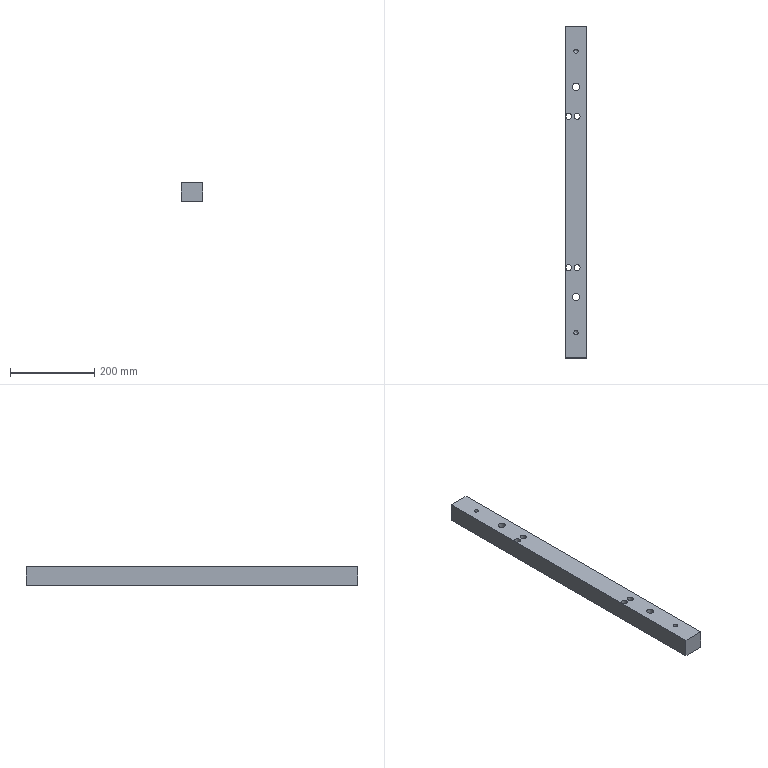Part | STEP file | 024_id2202_x_t | 1 solid | 20 faces | box 50 x 790 x 45 mm | volume 1716749 mm3 | cylinder 10 | plane 6 | cone 4 | commonest cylinder face diameters 14 x6 10.3 x2 17 x2